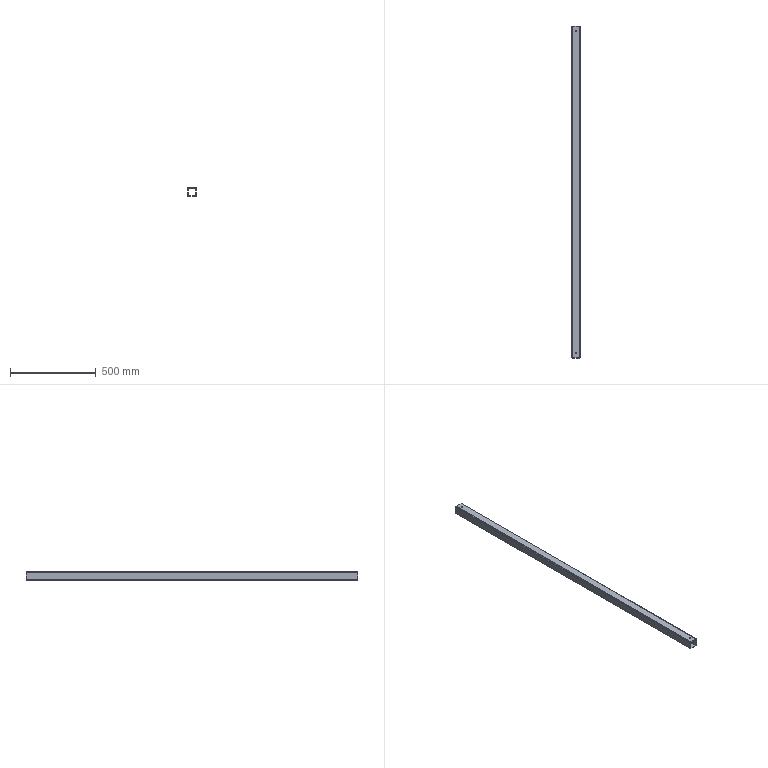Part | STEP file | POST.SQ.PIPE.1.stp | 1 solid | 30 faces | box 50 x 1940 x 50 mm | volume 1123447 mm3 | cylinder 18 | plane 10 | spline 2 | commonest cylinder face diameters 4 x8 10.4 x8 8 x2